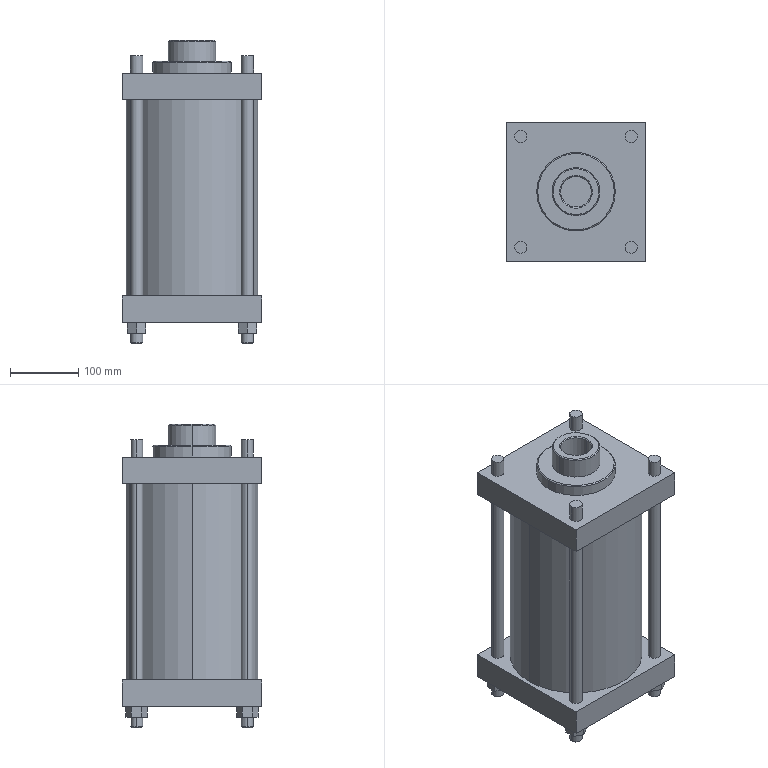Part | STEP file | CDS1FN180-250-A54Z_CS1-Body-1 | 1 solid | 129 faces | box 204 x 204 x 444 mm | volume 5555129 mm3 | plane 63 | cylinder 48 | cone 18 | commonest cylinder face diameters 18 x24 10.3 x6 17.7 x4 26.4 x4 45 x2 70 x2